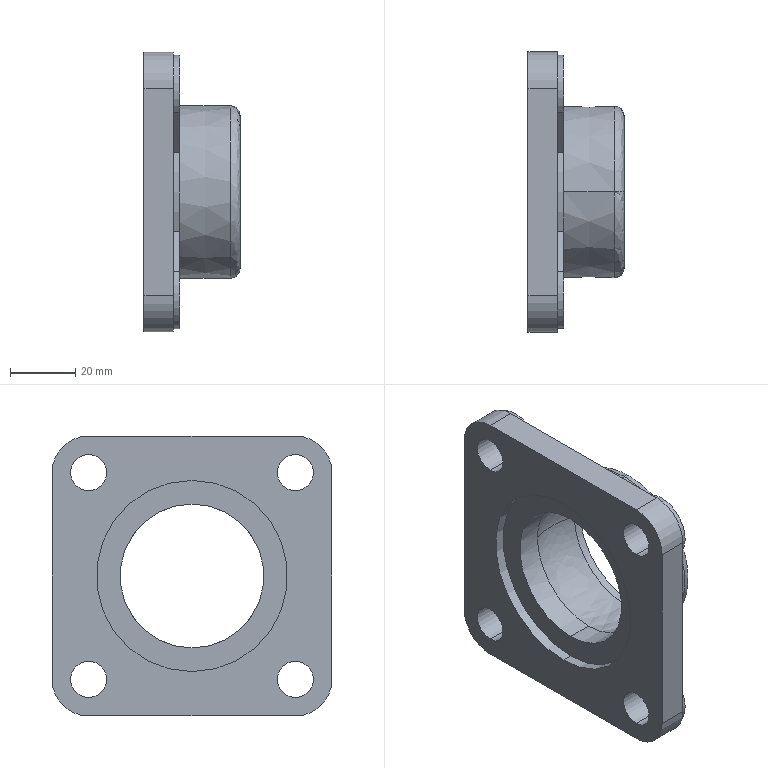Part | STEP file | Microwave Drying Flat Conveyor-FY 504 U_VA228_fyva_Default | 1 solid | 54 faces | box 29.5 x 86 x 86 mm | volume 59887 mm3 | cylinder 29 | plane 17 | spline 6 | cone 2 | commonest cylinder face diameters 11.1 x8 20.5 x6 22.5 x4 44.193 x4 58.362 x3 58.363 x2